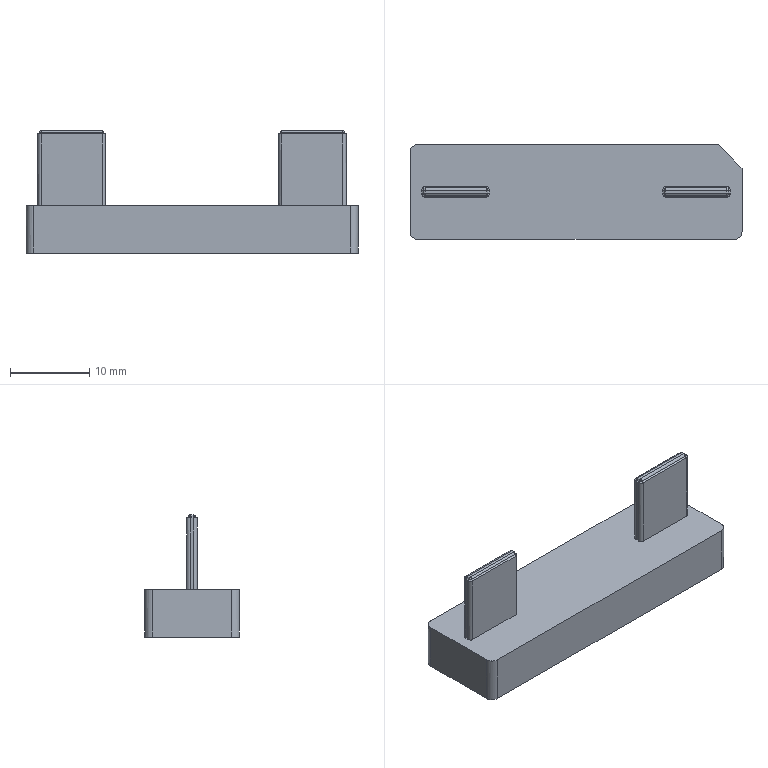NC program | PowerMill | posted with a generic post | part box 42 x 12 x 15.447 mm
Lines 9126 to 10040 of 88764:
N9223 M6
N9224 S8500 M03
N9225 G00 G90 X0.0 Y0.0
N9226 G43 Z11.797 H3
N9227
N9228 G05 P10000 R8
N9229 X-1.2399 Y3.9172
N9230 Z0.9272
N9231 G01 Z-0.2728 F360.0
N9232 X-6.1956 Y2.11 F600.0
N9233 X-24.3966 Y1.7747
N9234 X-24.4469 Y1.6032
N9235 X-24.5208 Y1.2816
N9236 X-24.5764 Y0.9594
N9237 X-24.6119 Y0.6374
N9238 X-24.6281 Y0.3163
N9239 X-24.6286 Y-0.3229
N9240 X-24.6005 Y-0.7367
N9241 X-24.571 Y-0.9658
N9242 X-24.5139 Y-1.288
N9243 X-24.4363 Y-1.6098
N9244 X-24.3134 Y-2.0045
N9245 X-24.2851 Y-2.0826
N9246 X-6.0837 Y-1.7473
N9247 G00 Z3.9972
N9248 G01 X29.1708 Y4.1105 F10000.0
N9249 G00 Z0.9272
N9250 G01 Z-0.2728 F360.0
N9251 X24.2541 Y2.1994 F600.0
N9252 X6.0642 Y1.7108
N9253 X6.0325 Y1.6032
N9254 X5.9585 Y1.2815
N9255 X5.9032 Y0.9595
N9256 X5.8675 Y0.6374
N9257 X5.851 Y0.3154
N9258 X5.8556 Y-0.322
N9259 X5.8748 Y-0.6441
N9260 X5.9132 Y-0.9658
N9261 X5.9703 Y-1.2883
N9262 X6.0694 Y-1.6927
N9263 X6.1437 Y-1.9314
N9264 X6.2304 Y-2.1674
N9265 X24.4162 Y-1.679
N9266 G00 Z11.797
N9267 G05 P0
N9268 (---------------)
N9269 ( END TOOLPATH : 精公基准台01-平坦面平行-D10 )
N9270 (---------------)
N9271 ( START TOOLPATH : 精公基准台01-基准面偏置-D10 )
N9272 (---------------)
N9273 G00 X0.0 Y0.0 Z9.7972
N9274 G05 P10000 R8
N9275 X31.7549 Y0.6644
N9276 Z-8.45
N9277 G01 Z-9.65 F360.0
N9278 X26.4799 Y0.6646 F600.0
N9279 X24.8744 Y0.57
N9280 X24.8826 Y0.3851
N9281 X24.8863 Y-0.0593
N9282 X24.8836 Y-0.3187
N9283 X24.8776 Y-0.4892
N9284 X24.8664 Y-0.6594
N9285 X24.8415 Y-0.9164
N9286 X24.8042 Y-1.1718
N9287 G02 X24.6105 Y-1.9836 I-5.5022 J0.8835
N9288 G01 X24.5391 Y-2.1973
N9289 X24.4587 Y-2.4078
N9290 X24.3431 Y-2.673
N9291 X24.2282 Y-2.9098
N9292 X24.1018 Y-3.1407
N9293 X23.9308 Y-3.417
N9294 X23.8088 Y-3.5975
N9295 X23.6776 Y-3.7754
N9296 X23.5455 Y-3.9406
N9297 X23.3966 Y-4.1135
N9298 X23.2404 Y-4.2799
N9299 X23.0219 Y-4.4915
N9300 X22.8267 Y-4.666
N9301 X22.6232 Y-4.8307
N9302 X22.4119 Y-4.9854
N9303 X22.1275 Y-5.1707
N9304 X21.8936 Y-5.3089
N9305 X21.6516 Y-5.4358
N9306 X21.461 Y-5.5251
N9307 X21.2115 Y-5.6291
N9308 X20.9575 Y-5.7231
N9309 X20.6992 Y-5.8041
N9310 X20.3792 Y-5.8856
N9311 X20.1129 Y-5.9405
N9312 X19.8442 Y-5.9818
N9313 X19.5144 Y-6.0141
N9314 X19.3078 Y-6.0261
N9315 X19.1008 Y-6.0301
N9316 X11.3792
N9317 G02 X10.8035 Y-5.9992 I0.0 J5.3801
N9318 G01 X10.4989 Y-5.9617
N9319 X10.2784 Y-5.9239
N9320 X10.0596 Y-5.877
N9321 X9.823 Y-5.8155
N9322 X9.5889 Y-5.7452
N9323 X9.3836 Y-5.674
N9324 X9.1814 Y-5.5944
N9325 X8.9819 Y-5.5084
N9326 G02 X8.3137 Y-5.1462 I2.2292 J4.9097
N9327 G01 X8.0573 Y-4.9774
N9328 X7.8773 Y-4.8463
N9329 X7.7029 Y-4.7079
N9330 X7.5214 Y-4.5507
N9331 X7.3458 Y-4.387
N9332 X7.1973 Y-4.2366
N9333 X7.0523 Y-4.0776
N9334 X6.9124 Y-3.9139
N9335 G02 X6.6038 Y-3.5 I4.2604 J3.4986
N9336 G01 X6.4784 Y-3.308
N9337 X6.3612 Y-3.111
N9338 X6.222 Y-2.8491
N9339 X6.1053 Y-2.6059
N9340 X6.001 Y-2.357
N9341 X5.8878 Y-2.039
N9342 X5.8231 Y-1.8308
N9343 X5.7653 Y-1.6138
N9344 G02 X5.658 Y-1.057 I5.5069 J1.35
N9345 G01 X5.628 Y-0.8223
N9346 X5.6051 Y-0.5335
N9347 X5.5955 Y-0.2759
N9348 X5.5938 Y0.0466
N9349 X5.5971 Y0.3691
N9350 X5.604 Y0.5443
N9351 X5.6161 Y0.7193
N9352 X5.6426 Y0.9784
N9353 X5.6732 Y1.1806
N9354 X0.9329 Y2.0168
N9355 G03 X0.8298 Y-1.0633 I10.7871 J-1.9028
N9356 G01 X0.8463 Y-1.2156
N9357 G03 X1.534 Y-4.0964 I11.6551 J1.26
N9358 G01 X1.6042 Y-4.2822
N9359 X1.8136 Y-4.7593
N9360 X2.228 Y-5.5966
N9361 G02 X1.5612 Y-6.6745 I-0.6668 J-0.3327
N9362 G01 X-1.5487
N9363 G02 X-2.2229 Y-5.5874 I0.0 J0.7526
N9364 G01 X-1.9073 Y-4.9511
N9365 G03 X-0.7717 Y-0.3011 I-9.7816 J4.8525
N9366 G01 X-0.7698 Y-0.2001
N9367 G03 X-1.8962 Y4.9213 I-11.2567 J0.2087
N9368 G01 X-2.2169 Y5.5825
N9369 G02 X-1.5336 Y6.6733 I0.6833 J0.3314
N9370 G01 X1.5263 Y6.6731
N9371 G02 X2.2038 Y5.585 I0.0 J-0.755
N9372 G01 X1.8898 Y4.9462
N9373 G03 X0.9329 Y2.0168 I9.8302 J-4.8322
N9374 G01 X5.6732 Y1.1806
N9375 X5.6816 Y1.2359
N9376 G02 X5.8729 Y2.0258 I5.4955 J-0.9132
N9377 G01 X5.944 Y2.2373
N9378 X6.0239 Y2.4456
N9379 X6.1393 Y2.7096
N9380 X6.2566 Y2.9507
N9381 X6.3858 Y3.1855
N9382 X6.5608 Y3.4663
N9383 X6.6844 Y3.6477
N9384 X6.8169 Y3.8261
N9385 X6.9429 Y3.9827
N9386 X7.0911 Y4.1539
N9387 X7.2463 Y4.3187
N9388 X7.4639 Y4.5289
N9389 X7.6599 Y4.7035
N9390 X7.8641 Y4.8683
N9391 X8.0761 Y5.023
N9392 X8.3614 Y5.2083
N9393 X8.5956 Y5.3461
N9394 X8.8376 Y5.4724
N9395 X9.0305 Y5.5624
N9396 X9.2831 Y5.6669
N9397 X9.5377 Y5.7604
N9398 X9.7967 Y5.8409
N9399 X10.1166 Y5.9214
N9400 X10.3797 Y5.9749
N9401 X10.6452 Y6.0153
N9402 X10.9124 Y6.0423
N9403 X11.1456 Y6.0572
N9404 X11.3792 Y6.0623
N9405 X19.1008
N9406 X19.3781 Y6.0551
N9407 X19.6546 Y6.0337
N9408 X19.9524 Y5.9984
N9409 X20.1697 Y5.9623
N9410 X20.3853 Y5.9174
N9411 X20.6233 Y5.857
N9412 X20.8588 Y5.7878
N9413 X21.069 Y5.7161
N9414 X21.2764 Y5.6356
N9415 X21.4811 Y5.5483
N9416 G02 X22.167 Y5.1778 I-2.2139 J-4.918
N9417 G01 X22.4391 Y4.9979
N9418 X22.6324 Y4.8555
N9419 X22.8191 Y4.7047
N9420 X22.9965 Y4.5473
N9421 X23.1674 Y4.3829
N9422 X23.3822 Y4.1599
N9423 X23.5234 Y3.9989
N9424 X23.6604 Y3.8295
N9425 X23.7699 Y3.6836
N9426 X23.8744 Y3.5342
N9427 X24.0012 Y3.3404
N9428 X24.1195 Y3.1414
N9429 X24.2587 Y2.8794
N9430 X24.372 Y2.6433
N9431 X24.4737 Y2.4019
N9432 X24.5845 Y2.0937
N9433 X24.6484 Y1.8913
N9434 X24.7058 Y1.6804
N9435 X24.758 Y1.452
N9436 X24.8008 Y1.2217
N9437 X24.8399 Y0.9582
N9438 X24.8744 Y0.57
N9439 X26.4799 Y0.6646
N9440 G00 Z2.8183
N9441 G01 X-31.7547 Y-0.5567 F10000.0
N9442 G00 Z-8.45
N9443 G01 Z-9.65 F360.0
N9444 X-26.4797 F600.0
N9445 X-24.876 Y-0.4924
N9446 X-24.8843 Y-0.2862
N9447 X-24.8862 Y0.0415
N9448 X-24.8829 Y0.3691
N9449 X-24.8761 Y0.5443
N9450 X-24.8639 Y0.7193
N9451 X-24.8374 Y0.9784
N9452 X-24.7984 Y1.2359
N9453 G02 X-24.6071 Y2.0258 I5.4937 J-0.9128
N9454 G01 X-24.536 Y2.2373
N9455 X-24.4561 Y2.4456
N9456 X-24.3407 Y2.7096
N9457 X-24.2234 Y2.9507
N9458 X-24.0942 Y3.1855
N9459 X-23.9192 Y3.4663
N9460 X-23.7956 Y3.6477
N9461 X-23.6631 Y3.8261
N9462 X-23.5371 Y3.9827
N9463 X-23.3889 Y4.1539
N9464 X-23.2337 Y4.3187
N9465 X-23.0161 Y4.5289
N9466 X-22.8201 Y4.7035
N9467 X-22.6159 Y4.8683
N9468 X-22.4039 Y5.023
N9469 X-22.1186 Y5.2083
N9470 X-21.8844 Y5.3461
N9471 X-21.6424 Y5.4724
N9472 X-21.4495 Y5.5624
N9473 X-21.1969 Y5.6669
N9474 X-20.9423 Y5.7604
N9475 X-20.6833 Y5.8409
N9476 X-20.3634 Y5.9214
N9477 X-20.1003 Y5.9749
N9478 X-19.8348 Y6.0153
N9479 X-19.5676 Y6.0423
N9480 X-19.3344 Y6.0572
N9481 X-19.1008 Y6.0623
N9482 X-11.3792
N9483 X-11.097 Y6.0549
N9484 X-10.8155 Y6.0327
N9485 X-10.515 Y5.9964
N9486 X-10.2965 Y5.9597
N9487 X-10.0797 Y5.9139
N9488 X-9.843 Y5.8533
N9489 X-9.6087 Y5.7838
N9490 X-9.4016 Y5.7127
N9491 X-9.1972 Y5.6331
N9492 X-8.9955 Y5.5468
N9493 X-8.8389 Y5.4731
N9494 X-8.5907 Y5.3434
N9495 X-8.2821 Y5.1586
N9496 X-8.0996 Y5.0391
N9497 X-7.9221 Y4.9122
N9498 X-7.7499 Y4.7783
N9499 X-7.5647 Y4.6211
N9500 X-7.3853 Y4.4572
N9501 X-7.2297 Y4.3023
N9502 X-7.0783 Y4.1386
N9503 X-6.9323 Y3.9699
N9504 X-6.8185 Y3.8281
N9505 X-6.6413 Y3.5865
N9506 X-6.5165 Y3.4002
N9507 X-6.3996 Y3.2089
N9508 X-6.2584 Y2.9516
N9509 X-6.1339 Y2.7003
N9510 X-6.0227 Y2.4429
N9511 X-5.9251 Y2.1801
N9512 X-5.8342 Y1.9
N9513 X-5.7735 Y1.6779
N9514 G02 X-5.6664 Y1.1429 I-5.4927 J-1.3787
N9515 G01 X-5.6336 Y0.9029
N9516 X-5.608 Y0.6075
N9517 X-5.5962 Y0.3305
N9518 X-5.5937 Y0.0059
N9519 X-5.5964 Y-0.3187
N9520 X-5.6024 Y-0.4892
N9521 X-5.6136 Y-0.6594
N9522 X-5.6385 Y-0.9164
N9523 X-5.6758 Y-1.1718
N9524 G02 X-5.8695 Y-1.9836 I-5.5033 J0.8838
N9525 G01 X-5.9409 Y-2.1973
N9526 X-6.0213 Y-2.4078
N9527 X-6.1369 Y-2.673
N9528 X-6.2518 Y-2.9098
N9529 X-6.3782 Y-3.1407
N9530 X-6.5492 Y-3.417
N9531 X-6.6712 Y-3.5975
N9532 X-6.8024 Y-3.7754
N9533 X-6.9345 Y-3.9406
N9534 X-7.0834 Y-4.1135
N9535 X-7.2396 Y-4.2799
N9536 X-7.4581 Y-4.4915
N9537 X-7.6533 Y-4.666
N9538 X-7.8568 Y-4.8307
N9539 X-8.0681 Y-4.9854
N9540 X-8.3525 Y-5.1707
N9541 X-8.5864 Y-5.3089
N9542 X-8.8284 Y-5.4358
N9543 X-9.019 Y-5.5251
N9544 X-9.2685 Y-5.6291
N9545 X-9.5225 Y-5.7231
N9546 X-9.7808 Y-5.8041
N9547 X-10.1008 Y-5.8856
N9548 X-10.3671 Y-5.9405
N9549 X-10.6358 Y-5.9818
N9550 X-10.9656 Y-6.0141
N9551 X-11.1722 Y-6.0261
N9552 X-11.3792 Y-6.0301
N9553 X-19.1008
N9554 G02 X-19.6836 Y-5.9984 I0.0 J5.3802
N9555 G01 X-19.9898 Y-5.9603
N9556 X-20.2111 Y-5.9221
N9557 X-20.4305 Y-5.8747
N9558 X-20.6658 Y-5.8131
N9559 X-20.8986 Y-5.7428
N9560 X-21.1012 Y-5.6722
N9561 G02 X-21.6519 Y-5.4356 I2.1624 J5.7939
N9562 G02 X-22.1893 Y-5.1315 I2.377 J4.8267
N9563 G01 X-22.4632 Y-4.9486
N9564 X-22.6566 Y-4.8046
N9565 X-22.8434 Y-4.6522
N9566 X-23.0232 Y-4.4915
N9567 X-23.2164 Y-4.3019
N9568 X-23.4025 Y-4.1054
N9569 X-23.5414 Y-3.9455
N9570 X-23.6763 Y-3.7771
N9571 X-23.7944 Y-3.6178
N9572 X-23.9067 Y-3.4543
N9573 X-24.0336 Y-3.256
N9574 X-24.1518 Y-3.0523
N9575 X-24.2891 Y-2.7868
N9576 X-24.3963 Y-2.5569
N9577 X-24.4925 Y-2.3222
N9578 X-24.5976 Y-2.0227
N9579 X-24.6589 Y-1.8241
N9580 X-24.7141 Y-1.6165
N9581 G02 X-24.8129 Y-1.1171 I5.4844 J1.3449
N9582 G01 X-24.8472 Y-0.8667
N9583 X-24.8733 Y-0.5612
N9584 X-24.876 Y-0.4924
N9585 X-26.4797 Y-0.5567
N9586 G00 Z9.7972
N9587 G05 P0
N9588 (---------------)
N9589 ( END TOOLPATH : 精公基准台01-基准面偏置-D10 )
N9590 (---------------)
N9591 ( START TOOLPATH : 精公基准台01-基准台侧光-D10 )
N9592 (---------------)
N9593 G00 X0.0 Y0.0 Z9.7972
N9594 G05 P10000 R8
N9595 X25.1661 Y-14.7991
N9596 Z-14.35
N9597 G01 Z-15.55 F360.0
N9598 G03 X22.8613 Y-10.362 I-1.1524 J2.2185 F600.0
N9599 G01 X22.6413 Y-10.4763
N9600 X22.6392 Y-10.4773
N9601 X22.6371 Y-10.4783
N9602 X22.3209 Y-10.6196
N9603 X22.3188 Y-10.6205
N9604 X22.3167 Y-10.6213
N9605 X22.0005 Y-10.7414
N9606 X21.9986 Y-10.7421
N9607 X21.9967 Y-10.7427
N9608 X21.742 Y-10.8251
N9609 X21.7399 Y-10.8257
N9610 X21.7378 Y-10.8263
N9611 X21.3602 Y-10.9258
N9612 X21.3578 Y-10.9264
N9613 X21.3554 Y-10.927
N9614 X21.0393 Y-10.9897
N9615 X21.0373 Y-10.9901
N9616 X21.0354 Y-10.9904
N9617 X20.7193 Y-11.0372
N9618 X20.717 Y-11.0375
N9619 X20.7147 Y-11.0377
N9620 X20.3985 Y-11.0661
N9621 X20.3966 Y-11.0662
N9622 X20.3947 Y-11.0663
N9623 X20.0786 Y-11.0794
N9624 X20.0769
N9625 X20.0753
N9626 X0.3161
N9627 X-20.0753
N9628 X-20.0768
N9629 X-20.0783
N9630 X-20.3945 Y-11.0672
N9631 X-20.3966 Y-11.0671
N9632 X-20.3987 Y-11.0669
N9633 X-20.7149 Y-11.0377
N9634 X-20.717 Y-11.0375
N9635 X-20.7191 Y-11.0372
N9636 X-21.0352 Y-10.9912
N9637 X-21.0373 Y-10.9909
N9638 X-21.0395 Y-10.9905
N9639 X-21.3556 Y-10.9269
N9640 X-21.3577 Y-10.9264
N9641 X-21.3598 Y-10.9259
N9642 X-21.676 Y-10.8443
N9643 X-21.6781 Y-10.8437
N9644 X-21.6802 Y-10.8431
N9645 X-21.9963 Y-10.7428
N9646 X-21.9984 Y-10.7421
N9647 X-22.0005 Y-10.7413
N9648 X-22.3167 Y-10.6213
N9649 X-22.3186 Y-10.6206
N9650 X-22.3205 Y-10.6197
N9651 X-22.5787 Y-10.506
N9652 X-22.5809 Y-10.505
N9653 X-22.583 Y-10.504
N9654 X-22.9571 Y-10.3122
N9655 X-22.959 Y-10.3112
N9656 X-22.9609 Y-10.3101
N9657 X-23.174 Y-10.1858
N9658 X-23.1751 Y-10.1851
N9659 X-23.1763 Y-10.1844
N9660 X-23.2793 Y-10.1196
N9661 X-23.2806 Y-10.1187
N9662 X-23.282 Y-10.1178
N9663 X-23.5981 Y-9.901
N9664 X-23.6003 Y-9.8994
N9665 X-23.6024 Y-9.8978
N9666 X-23.9185 Y-9.6488
N9667 X-23.92 Y-9.6476
N9668 X-23.9214 Y-9.6464
N9669 X-24.0386 Y-9.5448
N9670 X-24.0397 Y-9.5439
N9671 X-24.0408 Y-9.5429
N9672 X-24.2397 Y-9.3578
N9673 X-24.2408 Y-9.3567
N9674 X-24.2418 Y-9.3557
N9675 X-24.3723 Y-9.2247
N9676 X-24.3733 Y-9.2236
N9677 X-24.3744 Y-9.2225
N9678 X-24.5601 Y-9.0213
N9679 X-24.5611 Y-9.0202
N9680 X-24.5621 Y-9.019
N9681 X-24.6603 Y-8.904
N9682 X-24.6613 Y-8.9029
N9683 X-24.6622 Y-8.9017
N9684 X-24.8802 Y-8.6262
N9685 X-24.8818 Y-8.624
N9686 X-24.8834 Y-8.6219
N9687 X-25.1286 Y-8.2651
N9688 X-25.1297 Y-8.2636
N9689 X-25.1307 Y-8.262
N9690 X-25.2015 Y-8.1481
N9691 X-25.2022 Y-8.147
N9692 X-25.2029 Y-8.1458
N9693 X-25.3197 Y-7.9437
N9694 X-25.3206 Y-7.942
N9695 X-25.3215 Y-7.9403
N9696 X-25.4845 Y-7.6242
N9697 X-25.4856 Y-7.622
N9698 X-25.4866 Y-7.6199
N9699 X-25.6266 Y-7.3038
N9700 X-25.6275 Y-7.3017
N9701 X-25.6283 Y-7.2995
N9702 X-25.7474 Y-6.9834
N9703 X-25.7481 Y-6.9814
N9704 X-25.7488 Y-6.9793
N9705 X-25.8422 Y-6.6837
N9706 X-25.8428 Y-6.6816
N9707 X-25.8434 Y-6.6795
N9708 X-25.9298 Y-6.3428
N9709 X-25.9304 Y-6.3405
N9710 X-25.9308 Y-6.3383
N9711 X-25.9927 Y-6.0221
N9712 X-25.993 Y-6.0202
N9713 X-25.9933 Y-6.0183
N9714 X-26.0392 Y-5.7021
N9715 X-26.0395 Y-5.6998
N9716 X-26.0398 Y-5.6975
N9717 X-26.067 Y-5.3813
N9718 X-26.0672 Y-5.3795
N9719 X-26.0673 Y-5.3776
N9720 X-26.0796 Y-5.0615
N9721 Y-5.0599
N9722 X-26.0797 Y-5.0583
N9723 Y5.0583
N9724 Y5.0598
N9725 X-26.0796 Y5.0612
N9726 X-26.0683 Y5.3773
N9727 X-26.0682 Y5.3795
N9728 X-26.068 Y5.3816
N9729 X-26.0397 Y5.6977
N9730 X-26.0395 Y5.6998
N9731 X-26.0392 Y5.7019
N9732 X-25.9941 Y6.0181
N9733 X-25.9938 Y6.0202
N9734 X-25.9934 Y6.0223
N9735 X-25.9307 Y6.3385
N9736 X-25.9303 Y6.3406
N9737 X-25.9298 Y6.3427
N9738 X-25.8492 Y6.6588
N9739 X-25.8486 Y6.6609
N9740 X-25.848 Y6.663
N9741 X-25.7487 Y6.9792
N9742 X-25.748 Y6.9813
N9743 X-25.7473 Y6.9834
N9744 X-25.6283 Y7.2995
N9745 X-25.6275 Y7.3017
N9746 X-25.6266 Y7.3038
N9747 X-25.4865 Y7.6199
N9748 X-25.4855 Y7.622
N9749 X-25.4844 Y7.6241
N9750 X-25.3215 Y7.9403
N9751 X-25.3206 Y7.942
N9752 X-25.3197 Y7.9437
N9753 X-25.2029 Y8.1458
N9754 X-25.2022 Y8.147
N9755 X-25.2015 Y8.1481
N9756 X-25.1307 Y8.262
N9757 X-25.1298 Y8.2634
N9758 X-25.1288 Y8.2648
N9759 X-24.9135 Y8.581
N9760 X-24.912 Y8.5831
N9761 X-24.9104 Y8.5852
N9762 X-24.6632 Y8.9014
N9763 X-24.662 Y8.9028
N9764 X-24.6608 Y8.9042
N9765 X-24.562 Y9.0193
N9766 X-24.561 Y9.0204
N9767 X-24.5601 Y9.0214
N9768 X-24.3745 Y9.2225
N9769 X-24.3735 Y9.2236
N9770 X-24.3724 Y9.2247
N9771 X-24.2418 Y9.3557
N9772 X-24.2407 Y9.3567
N9773 X-24.2397 Y9.3578
N9774 X-24.0408 Y9.5429
N9775 X-24.0396 Y9.544
N9776 X-24.0384 Y9.545
N9777 X-23.9211 Y9.6458
N9778 X-23.92 Y9.6467
N9779 X-23.9189 Y9.6477
N9780 X-23.6491 Y9.863
N9781 X-23.647 Y9.8647
N9782 X-23.6448 Y9.8663
N9783 X-23.2823 Y10.1176
N9784 X-23.2808 Y10.1186
N9785 X-23.2793 Y10.1195
N9786 X-23.1763 Y10.1844
N9787 X-23.1751 Y10.1851
N9788 X-23.174 Y10.1858
N9789 X-22.9609 Y10.3101
N9790 X-22.9592 Y10.3111
N9791 X-22.9574 Y10.312
N9792 X-22.6413 Y10.4763
N9793 X-22.6392 Y10.4773
N9794 X-22.6371 Y10.4783
N9795 X-22.3209 Y10.6196
N9796 X-22.3188 Y10.6205
N9797 X-22.3167 Y10.6213
N9798 X-22.0005 Y10.7414
N9799 X-21.9986 Y10.7421
N9800 X-21.9967 Y10.7427
N9801 X-21.742 Y10.8251
N9802 X-21.7399 Y10.8257
N9803 X-21.7378 Y10.8263
N9804 X-21.3602 Y10.9258
N9805 X-21.3578 Y10.9264
N9806 X-21.3554 Y10.927
N9807 X-21.0393 Y10.9897
N9808 X-21.0373 Y10.9901
N9809 X-21.0354 Y10.9904
N9810 X-20.7193 Y11.0372
N9811 X-20.717 Y11.0375
N9812 X-20.7147 Y11.0377
N9813 X-20.3985 Y11.0661
N9814 X-20.3966 Y11.0662
N9815 X-20.3947 Y11.0663
N9816 X-20.0786 Y11.0794
N9817 X-20.0769
N9818 X-20.0753
N9819 X17.8622 Y11.08
N9820 X17.8626
N9821 X17.863
N9822 X18.1792 Y11.0768
N9823 X18.1815
N9824 X18.1838 Y11.0766
N9825 X18.4999 Y11.0553
N9826 X18.5024 Y11.0551
N9827 X18.505 Y11.0548
N9828 X18.8211 Y11.0132
N9829 X18.8237 Y11.0128
N9830 X18.8262 Y11.0123
N9831 X19.1423 Y10.9499
N9832 X19.1449 Y10.9493
N9833 X19.1474 Y10.9487
N9834 X19.4635 Y10.8646
N9835 X19.4653 Y10.8641
N9836 X19.467 Y10.8636
N9837 X19.5885 Y10.8252
N9838 X19.5898 Y10.8248
N9839 X19.591 Y10.8244
N9840 X19.7857 Y10.7558
N9841 X19.7878 Y10.755
N9842 X19.7898 Y10.7542
N9843 X20.1059 Y10.6229
N9844 X20.1085 Y10.6218
N9845 X20.111 Y10.6206
N9846 X20.4272 Y10.4626
N9847 X20.4297 Y10.4613
N9848 X20.4322 Y10.4598
N9849 X20.7484 Y10.2723
N9850 X20.7501 Y10.2712
N9851 X20.7519 Y10.2701
N9852 X20.8822 Y10.1832
N9853 X20.8835 Y10.1824
N9854 X20.8847 Y10.1815
N9855 X21.0706 Y10.0469
N9856 X21.0723 Y10.0457
N9857 X21.0739 Y10.0444
N9858 X21.2992 Y9.8628
N9859 X21.3005 Y9.8618
N9860 X21.3017 Y9.8607
N9861 X21.3925 Y9.7812
N9862 X21.3939 Y9.78
N9863 X21.3952 Y9.7787
N9864 X21.6421 Y9.5421
N9865 X21.6427 Y9.5415
N9866 X21.6433 Y9.5409
N9867 X24.5579 Y6.6264
N9868 X24.5586 Y6.6256
N9869 X24.5593 Y6.6249
N9870 X24.7941 Y6.378
N9871 X24.7953 Y6.3767
N9872 X24.7965 Y6.3753
N9873 X24.8779 Y6.2816
N9874 X24.8789 Y6.2803
N9875 X24.88 Y6.279
N9876 X25.0574 Y6.0567
N9877 X25.0587 Y6.055
N9878 X25.06 Y6.0533
N9879 X25.1986 Y5.8597
N9880 X25.1995 Y5.8584
N9881 X25.2004 Y5.8571
N9882 X25.2811 Y5.7347
N9883 X25.2822 Y5.7329
N9884 X25.2833 Y5.7312
N9885 X25.4692 Y5.415
N9886 X25.4701 Y5.4134
N9887 X25.471 Y5.4117
N9888 X25.5205 Y5.3176
N9889 X25.5212 Y5.3163
N9890 X25.5218 Y5.3151
N9891 X25.6288 Y5.0931
N9892 X25.6297 Y5.0909
N9893 X25.6307 Y5.0888
N9894 X25.7607 Y4.7726
N9895 X25.7616 Y4.7701
N9896 X25.7625 Y4.7675
N9897 X25.8682 Y4.4514
N9898 X25.869 Y4.4489
N9899 X25.8697 Y4.4463
N9900 X25.9526 Y4.1302
N9901 X25.9533 Y4.1277
N9902 X25.9538 Y4.1251
N9903 X26.0151 Y3.809
N9904 X26.0156 Y3.8065
N9905 X26.016 Y3.8039
N9906 X26.0565 Y3.4878
N9907 X26.0568 Y3.4853
N9908 X26.057 Y3.4827
N9909 X26.0772 Y3.1666
N9910 X26.0774 Y3.1643
N9911 Y3.1621
N9912 X26.08 Y2.846
N9913 Y2.8456
N9914 Y2.8453
N9915 X26.0797 Y-5.0583
N9916 Y-5.0598
N9917 X26.0796 Y-5.0612
N9918 X26.0683 Y-5.3773
N9919 X26.0681 Y-5.3795
N9920 X26.068 Y-5.3816
N9921 X26.0397 Y-5.6977
N9922 X26.0395 Y-5.6998
N9923 X26.0392 Y-5.7019
N9924 X25.9941 Y-6.0181
N9925 X25.9938 Y-6.0202
N9926 X25.9934 Y-6.0223
N9927 X25.9307 Y-6.3385
N9928 X25.9303 Y-6.3406
N9929 X25.9298 Y-6.3427
N9930 X25.8492 Y-6.6588
N9931 X25.8486 Y-6.6609
N9932 X25.848 Y-6.663
N9933 X25.7487 Y-6.9792
N9934 X25.748 Y-6.9813
N9935 X25.7473 Y-6.9834
N9936 X25.6283 Y-7.2995
N9937 X25.6275 Y-7.3017
N9938 X25.6266 Y-7.3038
N9939 X25.4865 Y-7.6199
N9940 X25.4855 Y-7.622
N9941 X25.4844 Y-7.6241
N9942 X25.3215 Y-7.9403
N9943 X25.3206 Y-7.942
N9944 X25.3197 Y-7.9437
N9945 X25.2029 Y-8.1458
N9946 X25.2022 Y-8.147
N9947 X25.2015 Y-8.1481
N9948 X25.1307 Y-8.262
N9949 X25.1298 Y-8.2634
N9950 X25.1288 Y-8.2648
N9951 X24.9135 Y-8.581
N9952 X24.912 Y-8.5831
N9953 X24.9104 Y-8.5852
N9954 X24.6632 Y-8.9014
N9955 X24.662 Y-8.9028
N9956 X24.6608 Y-8.9042
N9957 X24.562 Y-9.0193
N9958 X24.561 Y-9.0204
N9959 X24.5601 Y-9.0214
N9960 X24.3745 Y-9.2225
N9961 X24.3735 Y-9.2236
N9962 X24.3724 Y-9.2247
N9963 X24.2418 Y-9.3557
N9964 X24.2407 Y-9.3567
N9965 X24.2397 Y-9.3578
N9966 X24.0408 Y-9.5429
N9967 X24.0396 Y-9.544
N9968 X24.0384 Y-9.545
N9969 X23.9211 Y-9.6458
N9970 X23.92 Y-9.6467
N9971 X23.9189 Y-9.6477
N9972 X23.6491 Y-9.863
N9973 X23.647 Y-9.8647
N9974 X23.6448 Y-9.8663
N9975 X23.2823 Y-10.1176
N9976 X23.2808 Y-10.1186
N9977 X23.2793 Y-10.1195
N9978 X23.1763 Y-10.1844
N9979 X23.1751 Y-10.1851
N9980 X23.174 Y-10.1858
N9981 X22.9609 Y-10.3101
N9982 X22.9592 Y-10.3111
N9983 X22.9574 Y-10.312
N9984 X22.8613 Y-10.362
N9985 G03 X25.166 Y-14.7991 I1.1523 J-2.2186
N9986 G01 X25.1182 Y-14.7338
N9987 G03 X22.8134 Y-10.2967 I-1.1524 J2.2186
N9988 G01 X22.6044 Y-10.4053
N9989 X22.2883 Y-10.5465
N9990 X21.9721 Y-10.6666
N9991 X21.7174 Y-10.749
N9992 X21.3398 Y-10.8485
N9993 X21.0237 Y-10.9113
N9994 X20.7075 Y-10.9581
N9995 X20.3914 Y-10.9864
N9996 X20.0753 Y-10.9994
N9997 X19.7591 Y-11.0
N9998 X0.3161
N9999 X-19.1268
N10000 X-20.0753 Y-10.9994
N10001 X-20.3914 Y-10.9872
N10002 X-20.7075 Y-10.958
N10003 X-21.0237 Y-10.912
N10004 X-21.3398 Y-10.8484
N10005 X-21.656 Y-10.7668
N10006 X-21.9721 Y-10.6665
N10007 X-22.2883 Y-10.5465
N10008 X-22.5465 Y-10.4328
N10009 X-22.9206 Y-10.2411
N10010 X-23.1337 Y-10.1167
N10011 X-23.2367 Y-10.0519
N10012 X-23.5529 Y-9.835
N10013 X-23.869 Y-9.586
N10014 X-23.9862 Y-9.4844
N10015 X-24.1851 Y-9.2992
N10016 X-24.3156 Y-9.1682
N10017 X-24.5013 Y-8.9671
N10018 X-24.5995 Y-8.8521
N10019 X-24.8174 Y-8.5765
N10020 X-25.0627 Y-8.2198
N10021 X-25.1336 Y-8.1058
N10022 X-25.2504 Y-7.9036
N10023 X-25.4134 Y-7.5875
N10024 X-25.5535 Y-7.2714
N10025 X-25.6725 Y-6.9552
N10026 X-25.7659 Y-6.6596
N10027 X-25.8523 Y-6.3229
N10028 X-25.9142 Y-6.0068
N10029 X-25.9601 Y-5.6906
N10030 X-25.9873 Y-5.3745
N10031 X-25.9997 Y-5.0583
N10032 Y5.0583
N10033 X-25.9883 Y5.3745
N10034 X-25.9601 Y5.6906
N10035 X-25.9149 Y6.0068
N10036 X-25.8523 Y6.3229
N10037 X-25.7717 Y6.6391
N10038 X-25.6724 Y6.9552
N10039 X-25.5535 Y7.2714
N10040 X-25.4133 Y7.5875
N10041 X-25.2504 Y7.9036
N10042 X-25.1336 Y8.1058
N10043 X-25.0627 Y8.2198
N10044 X-24.8474 Y8.5359
N10045 X-24.6002 Y8.8521
N10046 X-24.5013 Y8.9672
N10047 X-24.3157 Y9.1682
N10048 X-24.1851 Y9.2992
N10049 X-23.9862 Y9.4844
N10050 X-23.869 Y9.5851
N10051 X-23.5992 Y9.8005
N10052 X-23.2367 Y10.0518
N10053 X-23.1337 Y10.1167
N10054 X-22.9206 Y10.2411
N10055 X-22.6044 Y10.4053
N10056 X-22.2883 Y10.5465
N10057 X-21.9721 Y10.6666
N10058 X-21.7174 Y10.749
N10059 X-21.3398 Y10.8485
N10060 X-21.0237 Y10.9113
N10061 X-20.7075 Y10.9581
N10062 X-20.3914 Y10.9864
N10063 X-20.0753 Y10.9994
N10064 X-19.7591 Y11.0
N10065 X17.8622
N10066 X18.1784 Y10.9968
N10067 X18.4945 Y10.9755
N10068 X18.8107 Y10.9339
N10069 X19.1268 Y10.8714
N10070 X19.443 Y10.7873
N10071 X19.5644 Y10.749
N10072 X19.7591 Y10.6803
N10073 X20.0753 Y10.549
N10074 X20.3914 Y10.391
N10075 X20.7075 Y10.2035
N10076 X20.8378 Y10.1167
N10077 X21.0237 Y9.9821
N10078 X21.249 Y9.8005
N10079 X21.3398 Y9.721
N10080 X21.5867 Y9.4844
N10081 X24.5013 Y6.5698
N10082 X24.7361 Y6.3229
N10083 X24.8174 Y6.2291
N10084 X24.9949 Y6.0068
N10085 X25.1336 Y5.8131
N10086 X25.2143 Y5.6906
N10087 X25.4002 Y5.3745
N10088 X25.4497 Y5.2803
N10089 X25.5567 Y5.0583
N10090 X25.6867 Y4.7422
N10091 X25.7923 Y4.426
N10092 X25.8753 Y4.1099
N10093 X25.9366 Y3.7937
N10094 X25.9772 Y3.4776
N10095 X25.9974 Y3.1615
N10096 X26.0 Y2.8453
N10097 X25.9997 Y-5.0583
N10098 X25.9883 Y-5.3745
N10099 X25.9601 Y-5.6906
N10100 X25.9149 Y-6.0068
N10101 X25.8523 Y-6.3229
N10102 X25.7717 Y-6.6391
N10103 X25.6724 Y-6.9552
N10104 X25.5535 Y-7.2714
N10105 X25.4133 Y-7.5875
N10106 X25.2504 Y-7.9036
N10107 X25.1336 Y-8.1058
N10108 X25.0627 Y-8.2198
N10109 X24.8474 Y-8.5359
N10110 X24.6002 Y-8.8521
N10111 X24.5013 Y-8.9672
N10112 X24.3157 Y-9.1682
N10113 X24.1851 Y-9.2992
N10114 X23.9862 Y-9.4844
N10115 X23.869 Y-9.5851
N10116 X23.5992 Y-9.8005
N10117 X23.2367 Y-10.0518
N10118 X23.1337 Y-10.1167
N10119 X22.9206 Y-10.2411
N10120 X22.8134 Y-10.2967
N10121 G03 X25.1182 Y-14.7338 I1.1524 J-2.2185
N10122 G00 Z9.7972
N10123 G05 P0
N10124 (---------------)
N10125 ( END TOOLPATH : 精公基准台01-基准台侧光-D10 )
N10126 (---------------)
N10127
N10128 M05
N10129 G53 Z0.0
N10130 (---------------)
N10131 ( START TOOLPATH : 精公精光01-等高-D4 )
N10132 (---------------)
N10133 ( TOOL NO.    :14 )
N10134 ( TOOL TYPE   : ENDMILL)
N10135 ( TOOL ID     : D4_1_1)
N10136 ( TOOL DIA    : 4.0 LENGTH 64.6)
N10137 T14